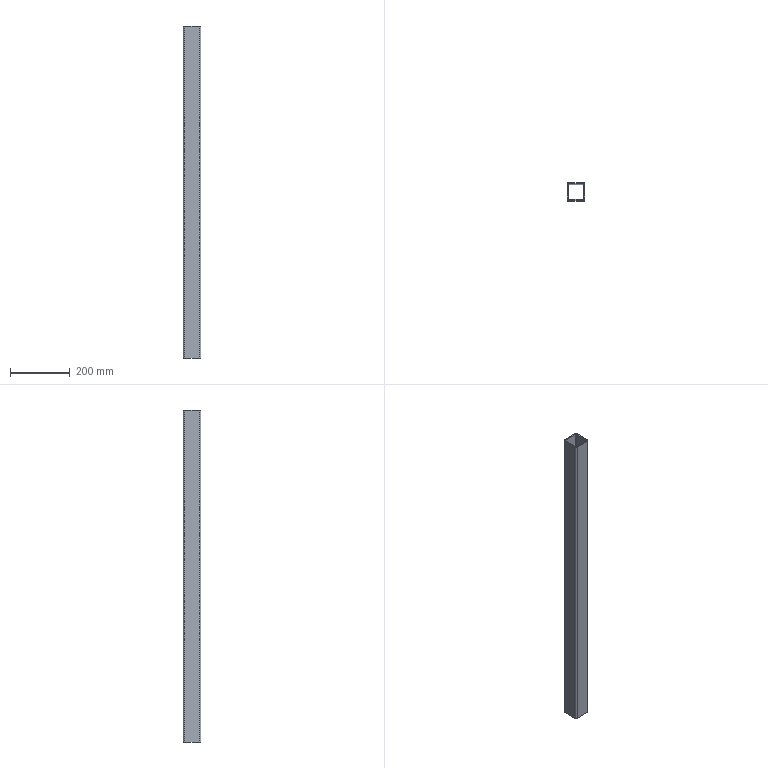Part | SolidWorks | features Extrusion 1, Fillet 1, Shell 1 | 1 solid | 18 faces | box 60 x 60 x 1116 mm | volume 976944 mm3 | plane 10 | cylinder 8 | commonest cylinder face diameters 2 x4 10 x4
STEP:
#1=CARTESIAN_POINT('',(-30.,25.,0.));
#2=VERTEX_POINT('',#1);
#3=CARTESIAN_POINT('',(-30.,-25.,0.));
#4=VERTEX_POINT('',#3);
#5=CARTESIAN_POINT('',(-30.,30.,0.));
#6=DIRECTION('',(0.,-1.,0.));
#7=VECTOR('',#6,1000.);
#8=LINE('',#5,#7);
#9=EDGE_CURVE('',#2,#4,#8,.T.);
#10=ORIENTED_EDGE('',*,*,#9,.F.);
#11=CARTESIAN_POINT('',(-25.,30.,0.));
#12=VERTEX_POINT('',#11);
#13=CARTESIAN_POINT('',(-25.,25.,0.));
#14=DIRECTION('',(0.,0.,-1.));
#15=DIRECTION('',(1.,0.,0.));
#16=AXIS2_PLACEMENT_3D('',#13,#14,#15);
#17=CIRCLE('',#16,5.);
#18=EDGE_CURVE('',#2,#12,#17,.T.);
#19=ORIENTED_EDGE('',*,*,#18,.T.);
#20=CARTESIAN_POINT('',(25.,30.,0.));
#21=VERTEX_POINT('',#20);
#22=CARTESIAN_POINT('',(30.,30.,0.));
#23=DIRECTION('',(-1.,0.,0.));
#24=VECTOR('',#23,1000.);
#25=LINE('',#22,#24);
#26=EDGE_CURVE('',#21,#12,#25,.T.);
#27=ORIENTED_EDGE('',*,*,#26,.F.);
#28=CARTESIAN_POINT('',(30.,25.,0.));
#29=VERTEX_POINT('',#28);
#30=CARTESIAN_POINT('',(25.,25.,0.));
#31=DIRECTION('',(0.,0.,-1.));
#32=DIRECTION('',(1.,0.,0.));
#33=AXIS2_PLACEMENT_3D('',#30,#31,#32);
#34=CIRCLE('',#33,5.);
#35=EDGE_CURVE('',#21,#29,#34,.T.);
#36=ORIENTED_EDGE('',*,*,#35,.T.);
#37=CARTESIAN_POINT('',(30.,-25.,0.));
#38=VERTEX_POINT('',#37);
#39=CARTESIAN_POINT('',(30.,30.,0.));
#40=DIRECTION('',(0.,-1.,0.));
#41=VECTOR('',#40,1000.);
#42=LINE('',#39,#41);
#43=EDGE_CURVE('',#29,#38,#42,.T.);
#44=ORIENTED_EDGE('',*,*,#43,.T.);
#45=CARTESIAN_POINT('',(25.,-30.,0.));
#46=VERTEX_POINT('',#45);
#47=CARTESIAN_POINT('',(25.,-25.,0.));
#48=DIRECTION('',(0.,0.,-1.));
#49=DIRECTION('',(1.,0.,0.));
#50=AXIS2_PLACEMENT_3D('',#47,#48,#49);
#51=CIRCLE('',#50,5.);
#52=EDGE_CURVE('',#38,#46,#51,.T.);
#53=ORIENTED_EDGE('',*,*,#52,.T.);
#54=CARTESIAN_POINT('',(-25.,-30.,0.));
#55=VERTEX_POINT('',#54);
#56=CARTESIAN_POINT('',(30.,-30.,0.));
#57=DIRECTION('',(-1.,0.,0.));
#58=VECTOR('',#57,1000.);
#59=LINE('',#56,#58);
#60=EDGE_CURVE('',#46,#55,#59,.T.);
#61=ORIENTED_EDGE('',*,*,#60,.T.);
#62=CARTESIAN_POINT('',(-25.,-25.,0.));
#63=DIRECTION('',(0.,0.,-1.));
#64=DIRECTION('',(1.,0.,0.));
#65=AXIS2_PLACEMENT_3D('',#62,#63,#64);
#66=CIRCLE('',#65,5.);
#67=EDGE_CURVE('',#55,#4,#66,.T.);
#68=ORIENTED_EDGE('',*,*,#67,.T.);
#69=EDGE_LOOP('',(#10,#19,#27,#36,#44,#53,#61,#68));
#70=FACE_OUTER_BOUND('',#69,.T.);
#71=CARTESIAN_POINT('',(-26.,25.,0.));
#72=VERTEX_POINT('',#71);
#73=CARTESIAN_POINT('',(-25.,26.,0.));
#74=VERTEX_POINT('',#73);
#75=CARTESIAN_POINT('',(-25.,25.,0.));
#76=DIRECTION('',(0.,0.,-1.));
#77=DIRECTION('',(1.,0.,0.));
#78=AXIS2_PLACEMENT_3D('',#75,#76,#77);
#79=CIRCLE('',#78,1.);
#80=EDGE_CURVE('',#72,#74,#79,.T.);
#81=ORIENTED_EDGE('',*,*,#80,.F.);
#82=CARTESIAN_POINT('',(-26.,-25.,0.));
#83=VERTEX_POINT('',#82);
#84=CARTESIAN_POINT('',(-26.,30.,0.));
#85=DIRECTION('',(0.,-1.,0.));
#86=VECTOR('',#85,1000.);
#87=LINE('',#84,#86);
#88=EDGE_CURVE('',#72,#83,#87,.T.);
#89=ORIENTED_EDGE('',*,*,#88,.T.);
#90=CARTESIAN_POINT('',(-25.,-26.,0.));
#91=VERTEX_POINT('',#90);
#92=CARTESIAN_POINT('',(-25.,-25.,0.));
#93=DIRECTION('',(0.,0.,-1.));
#94=DIRECTION('',(1.,0.,0.));
#95=AXIS2_PLACEMENT_3D('',#92,#93,#94);
#96=CIRCLE('',#95,1.);
#97=EDGE_CURVE('',#91,#83,#96,.T.);
#98=ORIENTED_EDGE('',*,*,#97,.F.);
#99=CARTESIAN_POINT('',(25.,-26.,0.));
#100=VERTEX_POINT('',#99);
#101=CARTESIAN_POINT('',(30.,-26.,0.));
#102=DIRECTION('',(-1.,0.,0.));
#103=VECTOR('',#102,1000.);
#104=LINE('',#101,#103);
#105=EDGE_CURVE('',#100,#91,#104,.T.);
#106=ORIENTED_EDGE('',*,*,#105,.F.);
#107=CARTESIAN_POINT('',(26.,-25.,0.));
#108=VERTEX_POINT('',#107);
#109=CARTESIAN_POINT('',(25.,-25.,0.));
#110=DIRECTION('',(0.,0.,-1.));
#111=DIRECTION('',(1.,0.,0.));
#112=AXIS2_PLACEMENT_3D('',#109,#110,#111);
#113=CIRCLE('',#112,1.);
#114=EDGE_CURVE('',#108,#100,#113,.T.);
#115=ORIENTED_EDGE('',*,*,#114,.F.);
#116=CARTESIAN_POINT('',(26.,25.,0.));
#117=VERTEX_POINT('',#116);
#118=CARTESIAN_POINT('',(26.,30.,0.));
#119=DIRECTION('',(0.,-1.,0.));
#120=VECTOR('',#119,1000.);
#121=LINE('',#118,#120);
#122=EDGE_CURVE('',#117,#108,#121,.T.);
#123=ORIENTED_EDGE('',*,*,#122,.F.);
#124=CARTESIAN_POINT('',(25.,26.,0.));
#125=VERTEX_POINT('',#124);
#126=CARTESIAN_POINT('',(25.,25.,0.));
#127=DIRECTION('',(0.,0.,-1.));
#128=DIRECTION('',(1.,0.,0.));
#129=AXIS2_PLACEMENT_3D('',#126,#127,#128);
#130=CIRCLE('',#129,1.);
#131=EDGE_CURVE('',#125,#117,#130,.T.);
#132=ORIENTED_EDGE('',*,*,#131,.F.);
#133=CARTESIAN_POINT('',(30.,26.,0.));
#134=DIRECTION('',(-1.,0.,0.));
#135=VECTOR('',#134,1000.);
#136=LINE('',#133,#135);
#137=EDGE_CURVE('',#125,#74,#136,.T.);
#138=ORIENTED_EDGE('',*,*,#137,.T.);
#139=EDGE_LOOP('',(#81,#89,#98,#106,#115,#123,#132,#138));
#140=FACE_BOUND('',#139,.T.);
#141=CARTESIAN_POINT('',(0.,0.,0.));
#142=DIRECTION('',(0.,0.,1.));
#143=DIRECTION('',(1.,0.,0.));
#144=AXIS2_PLACEMENT_3D('',#141,#142,#143);
#145=PLANE('',#144);
#146=ADVANCED_FACE('',(#70,#140),#145,.F.);
#147=ORIENTED_EDGE('',*,*,#60,.F.);
#148=CARTESIAN_POINT('',(25.,-30.,1116.));
#149=VERTEX_POINT('',#148);
#150=CARTESIAN_POINT('',(25.,-30.,1116.));
#151=DIRECTION('',(0.,0.,1.));
#152=VECTOR('',#151,1000.);
#153=LINE('',#150,#152);
#154=EDGE_CURVE('',#46,#149,#153,.T.);
#155=ORIENTED_EDGE('',*,*,#154,.T.);
#156=CARTESIAN_POINT('',(-25.,-30.,1116.));
#157=VERTEX_POINT('',#156);
#158=CARTESIAN_POINT('',(30.,-30.,1116.));
#159=DIRECTION('',(-1.,0.,0.));
#160=VECTOR('',#159,1000.);
#161=LINE('',#158,#160);
#162=EDGE_CURVE('',#149,#157,#161,.T.);
#163=ORIENTED_EDGE('',*,*,#162,.T.);
#164=CARTESIAN_POINT('',(-25.,-30.,0.));
#165=DIRECTION('',(0.,0.,-1.));
#166=VECTOR('',#165,1000.);
#167=LINE('',#164,#166);
#168=EDGE_CURVE('',#157,#55,#167,.T.);
#169=ORIENTED_EDGE('',*,*,#168,.T.);
#170=EDGE_LOOP('',(#147,#155,#163,#169));
#171=FACE_OUTER_BOUND('',#170,.T.);
#172=CARTESIAN_POINT('',(30.,-30.,1116.));
#173=DIRECTION('',(0.,-1.,0.));
#174=DIRECTION('',(1.,0.,0.));
#175=AXIS2_PLACEMENT_3D('',#172,#173,#174);
#176=PLANE('',#175);
#177=ADVANCED_FACE('',(#171),#176,.T.);
#178=ORIENTED_EDGE('',*,*,#43,.F.);
#179=CARTESIAN_POINT('',(30.,25.,1116.));
#180=VERTEX_POINT('',#179);
#181=CARTESIAN_POINT('',(30.,25.,1116.));
#182=DIRECTION('',(0.,0.,1.));
#183=VECTOR('',#182,1000.);
#184=LINE('',#181,#183);
#185=EDGE_CURVE('',#29,#180,#184,.T.);
#186=ORIENTED_EDGE('',*,*,#185,.T.);
#187=CARTESIAN_POINT('',(30.,-25.,1116.));
#188=VERTEX_POINT('',#187);
#189=CARTESIAN_POINT('',(30.,30.,1116.));
#190=DIRECTION('',(0.,-1.,0.));
#191=VECTOR('',#190,1000.);
#192=LINE('',#189,#191);
#193=EDGE_CURVE('',#180,#188,#192,.T.);
#194=ORIENTED_EDGE('',*,*,#193,.T.);
#195=CARTESIAN_POINT('',(30.,-25.,1116.));
#196=DIRECTION('',(0.,0.,-1.));
#197=VECTOR('',#196,1000.);
#198=LINE('',#195,#197);
#199=EDGE_CURVE('',#188,#38,#198,.T.);
#200=ORIENTED_EDGE('',*,*,#199,.T.);
#201=EDGE_LOOP('',(#178,#186,#194,#200));
#202=FACE_OUTER_BOUND('',#201,.T.);
#203=CARTESIAN_POINT('',(30.,30.,1116.));
#204=DIRECTION('',(1.,0.,0.));
#205=DIRECTION('',(0.,1.,0.));
#206=AXIS2_PLACEMENT_3D('',#203,#204,#205);
#207=PLANE('',#206);
#208=ADVANCED_FACE('',(#202),#207,.T.);
#209=ORIENTED_EDGE('',*,*,#26,.T.);
#210=CARTESIAN_POINT('',(-25.,30.,1116.));
#211=VERTEX_POINT('',#210);
#212=CARTESIAN_POINT('',(-25.,30.,1116.));
#213=DIRECTION('',(0.,0.,1.));
#214=VECTOR('',#213,1000.);
#215=LINE('',#212,#214);
#216=EDGE_CURVE('',#12,#211,#215,.T.);
#217=ORIENTED_EDGE('',*,*,#216,.T.);
#218=CARTESIAN_POINT('',(25.,30.,1116.));
#219=VERTEX_POINT('',#218);
#220=CARTESIAN_POINT('',(30.,30.,1116.));
#221=DIRECTION('',(-1.,0.,0.));
#222=VECTOR('',#221,1000.);
#223=LINE('',#220,#222);
#224=EDGE_CURVE('',#219,#211,#223,.T.);
#225=ORIENTED_EDGE('',*,*,#224,.F.);
#226=CARTESIAN_POINT('',(25.,30.,0.));
#227=DIRECTION('',(0.,0.,-1.));
#228=VECTOR('',#227,1000.);
#229=LINE('',#226,#228);
#230=EDGE_CURVE('',#219,#21,#229,.T.);
#231=ORIENTED_EDGE('',*,*,#230,.T.);
#232=EDGE_LOOP('',(#209,#217,#225,#231));
#233=FACE_OUTER_BOUND('',#232,.T.);
#234=CARTESIAN_POINT('',(30.,30.,1116.));
#235=DIRECTION('',(0.,-1.,0.));
#236=DIRECTION('',(1.,0.,0.));
#237=AXIS2_PLACEMENT_3D('',#234,#235,#236);
#238=PLANE('',#237);
#239=ADVANCED_FACE('',(#233),#238,.F.);
#240=CARTESIAN_POINT('',(-30.,25.,1116.));
#241=VERTEX_POINT('',#240);
#242=CARTESIAN_POINT('',(-30.,-25.,1116.));
#243=VERTEX_POINT('',#242);
#244=CARTESIAN_POINT('',(-30.,30.,1116.));
#245=DIRECTION('',(0.,-1.,0.));
#246=VECTOR('',#245,1000.);
#247=LINE('',#244,#246);
#248=EDGE_CURVE('',#241,#243,#247,.T.);
#249=ORIENTED_EDGE('',*,*,#248,.F.);
#250=CARTESIAN_POINT('',(-30.,25.,1116.));
#251=DIRECTION('',(0.,0.,-1.));
#252=VECTOR('',#251,1000.);
#253=LINE('',#250,#252);
#254=EDGE_CURVE('',#241,#2,#253,.T.);
#255=ORIENTED_EDGE('',*,*,#254,.T.);
#256=ORIENTED_EDGE('',*,*,#9,.T.);
#257=CARTESIAN_POINT('',(-30.,-25.,1116.));
#258=DIRECTION('',(0.,0.,1.));
#259=VECTOR('',#258,1000.);
#260=LINE('',#257,#259);
#261=EDGE_CURVE('',#4,#243,#260,.T.);
#262=ORIENTED_EDGE('',*,*,#261,.T.);
#263=EDGE_LOOP('',(#249,#255,#256,#262));
#264=FACE_OUTER_BOUND('',#263,.T.);
#265=CARTESIAN_POINT('',(-30.,30.,1116.));
#266=DIRECTION('',(1.,0.,0.));
#267=DIRECTION('',(0.,1.,0.));
#268=AXIS2_PLACEMENT_3D('',#265,#266,#267);
#269=PLANE('',#268);
#270=ADVANCED_FACE('',(#264),#269,.F.);
#271=CARTESIAN_POINT('',(25.,26.,1116.));
#272=VERTEX_POINT('',#271);
#273=CARTESIAN_POINT('',(-25.,26.,1116.));
#274=VERTEX_POINT('',#273);
#275=CARTESIAN_POINT('',(30.,26.,1116.));
#276=DIRECTION('',(-1.,0.,0.));
#277=VECTOR('',#276,1000.);
#278=LINE('',#275,#277);
#279=EDGE_CURVE('',#272,#274,#278,.T.);
#280=ORIENTED_EDGE('',*,*,#279,.F.);
#281=CARTESIAN_POINT('',(26.,25.,1116.));
#282=VERTEX_POINT('',#281);
#283=CARTESIAN_POINT('',(25.,25.,1116.));
#284=DIRECTION('',(0.,0.,1.));
#285=DIRECTION('',(1.,0.,0.));
#286=AXIS2_PLACEMENT_3D('',#283,#284,#285);
#287=CIRCLE('',#286,1.);
#288=EDGE_CURVE('',#282,#272,#287,.T.);
#289=ORIENTED_EDGE('',*,*,#288,.F.);
#290=CARTESIAN_POINT('',(26.,-25.,1116.));
#291=VERTEX_POINT('',#290);
#292=CARTESIAN_POINT('',(26.,30.,1116.));
#293=DIRECTION('',(0.,-1.,0.));
#294=VECTOR('',#293,1000.);
#295=LINE('',#292,#294);
#296=EDGE_CURVE('',#282,#291,#295,.T.);
#297=ORIENTED_EDGE('',*,*,#296,.T.);
#298=CARTESIAN_POINT('',(25.,-26.,1116.));
#299=VERTEX_POINT('',#298);
#300=CARTESIAN_POINT('',(25.,-25.,1116.));
#301=DIRECTION('',(0.,0.,1.));
#302=DIRECTION('',(1.,0.,0.));
#303=AXIS2_PLACEMENT_3D('',#300,#301,#302);
#304=CIRCLE('',#303,1.);
#305=EDGE_CURVE('',#299,#291,#304,.T.);
#306=ORIENTED_EDGE('',*,*,#305,.F.);
#307=CARTESIAN_POINT('',(-25.,-26.,1116.));
#308=VERTEX_POINT('',#307);
#309=CARTESIAN_POINT('',(30.,-26.,1116.));
#310=DIRECTION('',(-1.,0.,0.));
#311=VECTOR('',#310,1000.);
#312=LINE('',#309,#311);
#313=EDGE_CURVE('',#299,#308,#312,.T.);
#314=ORIENTED_EDGE('',*,*,#313,.T.);
#315=CARTESIAN_POINT('',(-26.,-25.,1116.));
#316=VERTEX_POINT('',#315);
#317=CARTESIAN_POINT('',(-25.,-25.,1116.));
#318=DIRECTION('',(0.,0.,1.));
#319=DIRECTION('',(1.,0.,0.));
#320=AXIS2_PLACEMENT_3D('',#317,#318,#319);
#321=CIRCLE('',#320,1.);
#322=EDGE_CURVE('',#316,#308,#321,.T.);
#323=ORIENTED_EDGE('',*,*,#322,.F.);
#324=CARTESIAN_POINT('',(-26.,25.,1116.));
#325=VERTEX_POINT('',#324);
#326=CARTESIAN_POINT('',(-26.,30.,1116.));
#327=DIRECTION('',(0.,-1.,0.));
#328=VECTOR('',#327,1000.);
#329=LINE('',#326,#328);
#330=EDGE_CURVE('',#325,#316,#329,.T.);
#331=ORIENTED_EDGE('',*,*,#330,.F.);
#332=CARTESIAN_POINT('',(-25.,25.,1116.));
#333=DIRECTION('',(0.,0.,1.));
#334=DIRECTION('',(1.,0.,0.));
#335=AXIS2_PLACEMENT_3D('',#332,#333,#334);
#336=CIRCLE('',#335,1.);
#337=EDGE_CURVE('',#274,#325,#336,.T.);
#338=ORIENTED_EDGE('',*,*,#337,.F.);
#339=EDGE_LOOP('',(#280,#289,#297,#306,#314,#323,#331,#338));
#340=FACE_BOUND('',#339,.T.);
#341=ORIENTED_EDGE('',*,*,#224,.T.);
#342=CARTESIAN_POINT('',(-25.,25.,1116.));
#343=DIRECTION('',(0.,0.,1.));
#344=DIRECTION('',(1.,0.,0.));
#345=AXIS2_PLACEMENT_3D('',#342,#343,#344);
#346=CIRCLE('',#345,5.);
#347=EDGE_CURVE('',#211,#241,#346,.T.);
#348=ORIENTED_EDGE('',*,*,#347,.T.);
#349=ORIENTED_EDGE('',*,*,#248,.T.);
#350=CARTESIAN_POINT('',(-25.,-25.,1116.));
#351=DIRECTION('',(0.,0.,1.));
#352=DIRECTION('',(1.,0.,0.));
#353=AXIS2_PLACEMENT_3D('',#350,#351,#352);
#354=CIRCLE('',#353,5.);
#355=EDGE_CURVE('',#243,#157,#354,.T.);
#356=ORIENTED_EDGE('',*,*,#355,.T.);
#357=ORIENTED_EDGE('',*,*,#162,.F.);
#358=CARTESIAN_POINT('',(25.,-25.,1116.));
#359=DIRECTION('',(0.,0.,1.));
#360=DIRECTION('',(1.,0.,0.));
#361=AXIS2_PLACEMENT_3D('',#358,#359,#360);
#362=CIRCLE('',#361,5.);
#363=EDGE_CURVE('',#149,#188,#362,.T.);
#364=ORIENTED_EDGE('',*,*,#363,.T.);
#365=ORIENTED_EDGE('',*,*,#193,.F.);
#366=CARTESIAN_POINT('',(25.,25.,1116.));
#367=DIRECTION('',(0.,0.,1.));
#368=DIRECTION('',(1.,0.,0.));
#369=AXIS2_PLACEMENT_3D('',#366,#367,#368);
#370=CIRCLE('',#369,5.);
#371=EDGE_CURVE('',#180,#219,#370,.T.);
#372=ORIENTED_EDGE('',*,*,#371,.T.);
#373=EDGE_LOOP('',(#341,#348,#349,#356,#357,#364,#365,#372));
#374=FACE_OUTER_BOUND('',#373,.T.);
#375=CARTESIAN_POINT('',(0.,0.,1116.));
#376=DIRECTION('',(0.,0.,1.));
#377=DIRECTION('',(1.,0.,0.));
#378=AXIS2_PLACEMENT_3D('',#375,#376,#377);
#379=PLANE('',#378);
#380=ADVANCED_FACE('',(#340,#374),#379,.T.);
#381=ORIENTED_EDGE('',*,*,#347,.F.);
#382=ORIENTED_EDGE('',*,*,#216,.F.);
#383=ORIENTED_EDGE('',*,*,#18,.F.);
#384=ORIENTED_EDGE('',*,*,#254,.F.);
#385=EDGE_LOOP('',(#381,#382,#383,#384));
#386=FACE_OUTER_BOUND('',#385,.T.);
#387=CARTESIAN_POINT('',(-25.,25.,1116.));
#388=DIRECTION('',(0.,0.,-1.));
#389=DIRECTION('',(-1.,0.,0.));
#390=AXIS2_PLACEMENT_3D('',#387,#388,#389);
#391=CYLINDRICAL_SURFACE('',#390,5.);
#392=ADVANCED_FACE('',(#386),#391,.T.);
#393=ORIENTED_EDGE('',*,*,#371,.F.);
#394=ORIENTED_EDGE('',*,*,#185,.F.);
#395=ORIENTED_EDGE('',*,*,#35,.F.);
#396=ORIENTED_EDGE('',*,*,#230,.F.);
#397=EDGE_LOOP('',(#393,#394,#395,#396));
#398=FACE_OUTER_BOUND('',#397,.T.);
#399=CARTESIAN_POINT('',(25.,25.,1116.));
#400=DIRECTION('',(0.,0.,1.));
#401=DIRECTION('',(1.,0.,0.));
#402=AXIS2_PLACEMENT_3D('',#399,#400,#401);
#403=CYLINDRICAL_SURFACE('',#402,5.);
#404=ADVANCED_FACE('',(#398),#403,.T.);
#405=ORIENTED_EDGE('',*,*,#363,.F.);
#406=ORIENTED_EDGE('',*,*,#154,.F.);
#407=ORIENTED_EDGE('',*,*,#52,.F.);
#408=ORIENTED_EDGE('',*,*,#199,.F.);
#409=EDGE_LOOP('',(#405,#406,#407,#408));
#410=FACE_OUTER_BOUND('',#409,.T.);
#411=CARTESIAN_POINT('',(25.,-25.,1116.));
#412=DIRECTION('',(0.,0.,-1.));
#413=DIRECTION('',(-1.,0.,0.));
#414=AXIS2_PLACEMENT_3D('',#411,#412,#413);
#415=CYLINDRICAL_SURFACE('',#414,5.);
#416=ADVANCED_FACE('',(#410),#415,.T.);
#417=ORIENTED_EDGE('',*,*,#355,.F.);
#418=ORIENTED_EDGE('',*,*,#261,.F.);
#419=ORIENTED_EDGE('',*,*,#67,.F.);
#420=ORIENTED_EDGE('',*,*,#168,.F.);
#421=EDGE_LOOP('',(#417,#418,#419,#420));
#422=FACE_OUTER_BOUND('',#421,.T.);
#423=CARTESIAN_POINT('',(-25.,-25.,1116.));
#424=DIRECTION('',(0.,0.,1.));
#425=DIRECTION('',(1.,0.,0.));
#426=AXIS2_PLACEMENT_3D('',#423,#424,#425);
#427=CYLINDRICAL_SURFACE('',#426,5.);
#428=ADVANCED_FACE('',(#422),#427,.T.);
#429=ORIENTED_EDGE('',*,*,#105,.T.);
#430=CARTESIAN_POINT('',(-25.,-26.,1116.));
#431=DIRECTION('',(0.,0.,-1.));
#432=VECTOR('',#431,1000.);
#433=LINE('',#430,#432);
#434=EDGE_CURVE('',#308,#91,#433,.T.);
#435=ORIENTED_EDGE('',*,*,#434,.F.);
#436=ORIENTED_EDGE('',*,*,#313,.F.);
#437=CARTESIAN_POINT('',(25.,-26.,1116.));
#438=DIRECTION('',(0.,0.,1.));
#439=VECTOR('',#438,1000.);
#440=LINE('',#437,#439);
#441=EDGE_CURVE('',#100,#299,#440,.T.);
#442=ORIENTED_EDGE('',*,*,#441,.F.);
#443=EDGE_LOOP('',(#429,#435,#436,#442));
#444=FACE_OUTER_BOUND('',#443,.T.);
#445=CARTESIAN_POINT('',(30.,-26.,1116.));
#446=DIRECTION('',(0.,-1.,0.));
#447=DIRECTION('',(1.,0.,0.));
#448=AXIS2_PLACEMENT_3D('',#445,#446,#447);
#449=PLANE('',#448);
#450=ADVANCED_FACE('',(#444),#449,.F.);
#451=ORIENTED_EDGE('',*,*,#122,.T.);
#452=CARTESIAN_POINT('',(26.,-25.,1116.));
#453=DIRECTION('',(0.,0.,-1.));
#454=VECTOR('',#453,1000.);
#455=LINE('',#452,#454);
#456=EDGE_CURVE('',#291,#108,#455,.T.);
#457=ORIENTED_EDGE('',*,*,#456,.F.);
#458=ORIENTED_EDGE('',*,*,#296,.F.);
#459=CARTESIAN_POINT('',(26.,25.,1116.));
#460=DIRECTION('',(0.,0.,1.));
#461=VECTOR('',#460,1000.);
#462=LINE('',#459,#461);
#463=EDGE_CURVE('',#117,#282,#462,.T.);
#464=ORIENTED_EDGE('',*,*,#463,.F.);
#465=EDGE_LOOP('',(#451,#457,#458,#464));
#466=FACE_OUTER_BOUND('',#465,.T.);
#467=CARTESIAN_POINT('',(26.,30.,1116.));
#468=DIRECTION('',(1.,0.,0.));
#469=DIRECTION('',(0.,1.,0.));
#470=AXIS2_PLACEMENT_3D('',#467,#468,#469);
#471=PLANE('',#470);
#472=ADVANCED_FACE('',(#466),#471,.F.);
#473=ORIENTED_EDGE('',*,*,#137,.F.);
#474=CARTESIAN_POINT('',(25.,26.,1116.));
#475=DIRECTION('',(0.,0.,-1.));
#476=VECTOR('',#475,1000.);
#477=LINE('',#474,#476);
#478=EDGE_CURVE('',#272,#125,#477,.T.);
#479=ORIENTED_EDGE('',*,*,#478,.F.);
#480=ORIENTED_EDGE('',*,*,#279,.T.);
#481=CARTESIAN_POINT('',(-25.,26.,1116.));
#482=DIRECTION('',(0.,0.,1.));
#483=VECTOR('',#482,1000.);
#484=LINE('',#481,#483);
#485=EDGE_CURVE('',#74,#274,#484,.T.);
#486=ORIENTED_EDGE('',*,*,#485,.F.);
#487=EDGE_LOOP('',(#473,#479,#480,#486));
#488=FACE_OUTER_BOUND('',#487,.T.);
#489=CARTESIAN_POINT('',(30.,26.,1116.));
#490=DIRECTION('',(0.,-1.,0.));
#491=DIRECTION('',(1.,0.,0.));
#492=AXIS2_PLACEMENT_3D('',#489,#490,#491);
#493=PLANE('',#492);
#494=ADVANCED_FACE('',(#488),#493,.T.);
#495=ORIENTED_EDGE('',*,*,#330,.T.);
#496=CARTESIAN_POINT('',(-26.,-25.,1116.));
#497=DIRECTION('',(0.,0.,1.));
#498=VECTOR('',#497,1000.);
#499=LINE('',#496,#498);
#500=EDGE_CURVE('',#83,#316,#499,.T.);
#501=ORIENTED_EDGE('',*,*,#500,.F.);
#502=ORIENTED_EDGE('',*,*,#88,.F.);
#503=CARTESIAN_POINT('',(-26.,25.,1116.));
#504=DIRECTION('',(0.,0.,-1.));
#505=VECTOR('',#504,1000.);
#506=LINE('',#503,#505);
#507=EDGE_CURVE('',#325,#72,#506,.T.);
#508=ORIENTED_EDGE('',*,*,#507,.F.);
#509=EDGE_LOOP('',(#495,#501,#502,#508));
#510=FACE_OUTER_BOUND('',#509,.T.);
#511=CARTESIAN_POINT('',(-26.,30.,1116.));
#512=DIRECTION('',(1.,0.,0.));
#513=DIRECTION('',(0.,1.,0.));
#514=AXIS2_PLACEMENT_3D('',#511,#512,#513);
#515=PLANE('',#514);
#516=ADVANCED_FACE('',(#510),#515,.T.);
#517=ORIENTED_EDGE('',*,*,#337,.T.);
#518=ORIENTED_EDGE('',*,*,#507,.T.);
#519=ORIENTED_EDGE('',*,*,#80,.T.);
#520=ORIENTED_EDGE('',*,*,#485,.T.);
#521=EDGE_LOOP('',(#517,#518,#519,#520));
#522=FACE_OUTER_BOUND('',#521,.T.);
#523=CARTESIAN_POINT('',(-25.,25.,1116.));
#524=DIRECTION('',(0.,0.,-1.));
#525=DIRECTION('',(-1.,0.,0.));
#526=AXIS2_PLACEMENT_3D('',#523,#524,#525);
#527=CYLINDRICAL_SURFACE('',#526,1.);
#528=ADVANCED_FACE('',(#522),#527,.F.);
#529=ORIENTED_EDGE('',*,*,#288,.T.);
#530=ORIENTED_EDGE('',*,*,#478,.T.);
#531=ORIENTED_EDGE('',*,*,#131,.T.);
#532=ORIENTED_EDGE('',*,*,#463,.T.);
#533=EDGE_LOOP('',(#529,#530,#531,#532));
#534=FACE_OUTER_BOUND('',#533,.T.);
#535=CARTESIAN_POINT('',(25.,25.,1116.));
#536=DIRECTION('',(0.,0.,1.));
#537=DIRECTION('',(1.,0.,0.));
#538=AXIS2_PLACEMENT_3D('',#535,#536,#537);
#539=CYLINDRICAL_SURFACE('',#538,1.);
#540=ADVANCED_FACE('',(#534),#539,.F.);
#541=ORIENTED_EDGE('',*,*,#305,.T.);
#542=ORIENTED_EDGE('',*,*,#456,.T.);
#543=ORIENTED_EDGE('',*,*,#114,.T.);
#544=ORIENTED_EDGE('',*,*,#441,.T.);
#545=EDGE_LOOP('',(#541,#542,#543,#544));
#546=FACE_OUTER_BOUND('',#545,.T.);
#547=CARTESIAN_POINT('',(25.,-25.,1116.));
#548=DIRECTION('',(0.,0.,-1.));
#549=DIRECTION('',(-1.,0.,0.));
#550=AXIS2_PLACEMENT_3D('',#547,#548,#549);
#551=CYLINDRICAL_SURFACE('',#550,1.);
#552=ADVANCED_FACE('',(#546),#551,.F.);
#553=ORIENTED_EDGE('',*,*,#322,.T.);
#554=ORIENTED_EDGE('',*,*,#434,.T.);
#555=ORIENTED_EDGE('',*,*,#97,.T.);
#556=ORIENTED_EDGE('',*,*,#500,.T.);
#557=EDGE_LOOP('',(#553,#554,#555,#556));
#558=FACE_OUTER_BOUND('',#557,.T.);
#559=CARTESIAN_POINT('',(-25.,-25.,1116.));
#560=DIRECTION('',(0.,0.,1.));
#561=DIRECTION('',(1.,0.,0.));
#562=AXIS2_PLACEMENT_3D('',#559,#560,#561);
#563=CYLINDRICAL_SURFACE('',#562,1.);
#564=ADVANCED_FACE('',(#558),#563,.F.);
#565=CLOSED_SHELL('',(#146,#177,#208,#239,#270,#380,#392,#404,#416,#428,#450,#472,#494,#516,#528,#540,#552,#564));
#566=MANIFOLD_SOLID_BREP('',#565);
#567=CARTESIAN_POINT('',(0.,0.,0.));
#568=DIRECTION('',(0.,0.,1.));
#569=DIRECTION('',(1.,0.,0.));
#570=AXIS2_PLACEMENT_3D('',#567,#568,#569);
#571=(LENGTH_UNIT()NAMED_UNIT(*)SI_UNIT(.MILLI.,.METRE.));
#572=UNCERTAINTY_MEASURE_WITH_UNIT(LENGTH_MEASURE(0.00001),#571,'','');
#573=(NAMED_UNIT(*)PLANE_ANGLE_UNIT()SI_UNIT($,.RADIAN.));
#574=(NAMED_UNIT(*)SI_UNIT($,.STERADIAN.)SOLID_ANGLE_UNIT());
#575=(GEOMETRIC_REPRESENTATION_CONTEXT(3)GLOBAL_UNCERTAINTY_ASSIGNED_CONTEXT((#572))GLOBAL_UNIT_ASSIGNED_CONTEXT((#571,#573,#574))REPRESENTATION_CONTEXT('',''));
#576=ADVANCED_BREP_SHAPE_REPRESENTATION('',(#566,#570),#575);